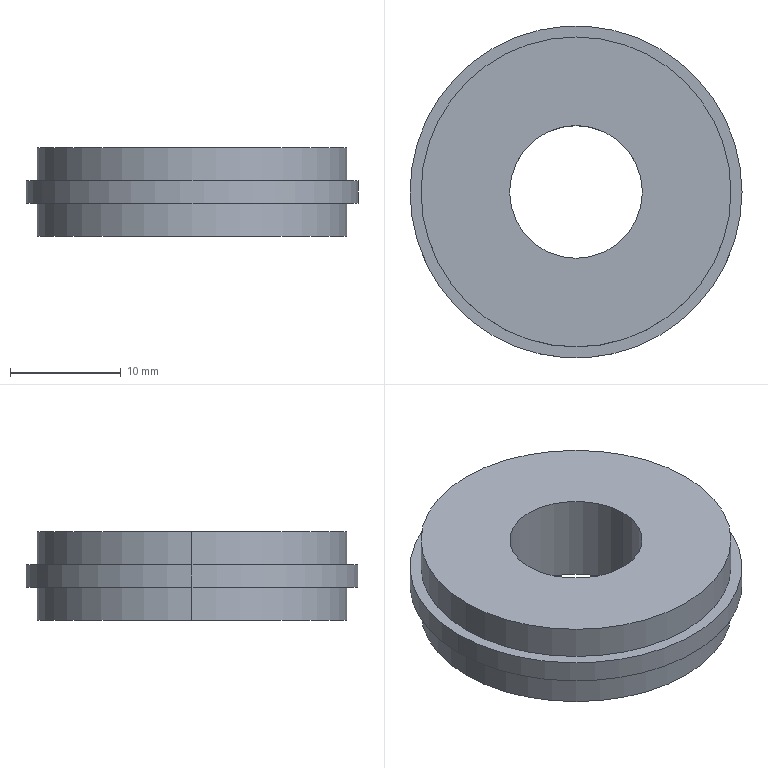Part | SolidWorks | features BaseBody 1 | 1 solid | 12 faces | box 30 x 30 x 8 mm | volume 4203 mm3 | cylinder 8 | plane 4 | commonest cylinder face diameters 28 x4 12 x2 30 x2
STEP:
#1=CARTESIAN_POINT('',(6.,0.,4.));
#2=VERTEX_POINT('',#1);
#3=CARTESIAN_POINT('',(-6.,0.,4.));
#4=VERTEX_POINT('',#3);
#5=CARTESIAN_POINT('',(0.,0.,4.));
#6=DIRECTION('',(0.,0.,-1.));
#7=DIRECTION('',(-1.,0.,0.));
#8=AXIS2_PLACEMENT_3D('',#5,#6,#7);
#9=CIRCLE('',#8,6.);
#10=EDGE_CURVE('',#2,#4,#9,.T.);
#11=ORIENTED_EDGE('',*,*,#10,.F.);
#12=CARTESIAN_POINT('',(6.,0.,-4.));
#13=VERTEX_POINT('',#12);
#14=CARTESIAN_POINT('',(6.,0.,4.));
#15=DIRECTION('',(0.,0.,-1.));
#16=VECTOR('',#15,1000.);
#17=LINE('',#14,#16);
#18=EDGE_CURVE('',#2,#13,#17,.T.);
#19=ORIENTED_EDGE('',*,*,#18,.T.);
#20=CARTESIAN_POINT('',(-6.,0.,-4.));
#21=VERTEX_POINT('',#20);
#22=CARTESIAN_POINT('',(0.,0.,-4.));
#23=DIRECTION('',(0.,0.,-1.));
#24=DIRECTION('',(-1.,0.,0.));
#25=AXIS2_PLACEMENT_3D('',#22,#23,#24);
#26=CIRCLE('',#25,6.);
#27=EDGE_CURVE('',#13,#21,#26,.T.);
#28=ORIENTED_EDGE('',*,*,#27,.T.);
#29=CARTESIAN_POINT('',(-6.,0.,4.));
#30=DIRECTION('',(0.,0.,-1.));
#31=VECTOR('',#30,1000.);
#32=LINE('',#29,#31);
#33=EDGE_CURVE('',#4,#21,#32,.T.);
#34=ORIENTED_EDGE('',*,*,#33,.F.);
#35=EDGE_LOOP('',(#11,#19,#28,#34));
#36=FACE_OUTER_BOUND('',#35,.T.);
#37=CARTESIAN_POINT('',(0.,0.,4.));
#38=DIRECTION('',(0.,0.,-1.));
#39=DIRECTION('',(-1.,0.,0.));
#40=AXIS2_PLACEMENT_3D('',#37,#38,#39);
#41=CYLINDRICAL_SURFACE('',#40,6.);
#42=ADVANCED_FACE('',(#36),#41,.F.);
#43=CARTESIAN_POINT('',(14.,0.,-4.));
#44=VERTEX_POINT('',#43);
#45=CARTESIAN_POINT('',(-14.,0.,-4.));
#46=VERTEX_POINT('',#45);
#47=CARTESIAN_POINT('',(0.,0.,-4.));
#48=DIRECTION('',(0.,0.,1.));
#49=DIRECTION('',(1.,0.,0.));
#50=AXIS2_PLACEMENT_3D('',#47,#48,#49);
#51=CIRCLE('',#50,14.);
#52=EDGE_CURVE('',#44,#46,#51,.T.);
#53=ORIENTED_EDGE('',*,*,#52,.T.);
#54=CARTESIAN_POINT('',(-14.,0.,-1.));
#55=VERTEX_POINT('',#54);
#56=CARTESIAN_POINT('',(-14.,0.,-4.));
#57=DIRECTION('',(0.,0.,1.));
#58=VECTOR('',#57,1000.);
#59=LINE('',#56,#58);
#60=EDGE_CURVE('',#46,#55,#59,.T.);
#61=ORIENTED_EDGE('',*,*,#60,.T.);
#62=CARTESIAN_POINT('',(14.,0.,-1.));
#63=VERTEX_POINT('',#62);
#64=CARTESIAN_POINT('',(0.,0.,-1.));
#65=DIRECTION('',(0.,0.,1.));
#66=DIRECTION('',(1.,0.,0.));
#67=AXIS2_PLACEMENT_3D('',#64,#65,#66);
#68=CIRCLE('',#67,14.);
#69=EDGE_CURVE('',#63,#55,#68,.T.);
#70=ORIENTED_EDGE('',*,*,#69,.F.);
#71=CARTESIAN_POINT('',(14.,0.,-4.));
#72=DIRECTION('',(0.,0.,1.));
#73=VECTOR('',#72,1000.);
#74=LINE('',#71,#73);
#75=EDGE_CURVE('',#44,#63,#74,.T.);
#76=ORIENTED_EDGE('',*,*,#75,.F.);
#77=EDGE_LOOP('',(#53,#61,#70,#76));
#78=FACE_OUTER_BOUND('',#77,.T.);
#79=CARTESIAN_POINT('',(0.,0.,-4.));
#80=DIRECTION('',(0.,0.,1.));
#81=DIRECTION('',(1.,0.,0.));
#82=AXIS2_PLACEMENT_3D('',#79,#80,#81);
#83=CYLINDRICAL_SURFACE('',#82,14.);
#84=ADVANCED_FACE('',(#78),#83,.T.);
#85=CARTESIAN_POINT('',(14.,0.,4.));
#86=VERTEX_POINT('',#85);
#87=CARTESIAN_POINT('',(-14.,0.,4.));
#88=VERTEX_POINT('',#87);
#89=CARTESIAN_POINT('',(0.,0.,4.));
#90=DIRECTION('',(0.,0.,1.));
#91=DIRECTION('',(1.,0.,0.));
#92=AXIS2_PLACEMENT_3D('',#89,#90,#91);
#93=CIRCLE('',#92,14.);
#94=EDGE_CURVE('',#86,#88,#93,.T.);
#95=ORIENTED_EDGE('',*,*,#94,.F.);
#96=CARTESIAN_POINT('',(14.,0.,1.));
#97=VERTEX_POINT('',#96);
#98=CARTESIAN_POINT('',(14.,0.,4.));
#99=DIRECTION('',(0.,0.,-1.));
#100=VECTOR('',#99,1000.);
#101=LINE('',#98,#100);
#102=EDGE_CURVE('',#86,#97,#101,.T.);
#103=ORIENTED_EDGE('',*,*,#102,.T.);
#104=CARTESIAN_POINT('',(-14.,0.,1.));
#105=VERTEX_POINT('',#104);
#106=CARTESIAN_POINT('',(0.,0.,1.));
#107=DIRECTION('',(0.,0.,1.));
#108=DIRECTION('',(1.,0.,0.));
#109=AXIS2_PLACEMENT_3D('',#106,#107,#108);
#110=CIRCLE('',#109,14.);
#111=EDGE_CURVE('',#97,#105,#110,.T.);
#112=ORIENTED_EDGE('',*,*,#111,.T.);
#113=CARTESIAN_POINT('',(-14.,0.,4.));
#114=DIRECTION('',(0.,0.,-1.));
#115=VECTOR('',#114,1000.);
#116=LINE('',#113,#115);
#117=EDGE_CURVE('',#88,#105,#116,.T.);
#118=ORIENTED_EDGE('',*,*,#117,.F.);
#119=EDGE_LOOP('',(#95,#103,#112,#118));
#120=FACE_OUTER_BOUND('',#119,.T.);
#121=CARTESIAN_POINT('',(0.,0.,4.));
#122=DIRECTION('',(0.,0.,-1.));
#123=DIRECTION('',(-1.,0.,0.));
#124=AXIS2_PLACEMENT_3D('',#121,#122,#123);
#125=CYLINDRICAL_SURFACE('',#124,14.);
#126=ADVANCED_FACE('',(#120),#125,.T.);
#127=CARTESIAN_POINT('',(15.,0.,1.));
#128=VERTEX_POINT('',#127);
#129=CARTESIAN_POINT('',(-15.,0.,1.));
#130=VERTEX_POINT('',#129);
#131=CARTESIAN_POINT('',(0.,0.,1.));
#132=DIRECTION('',(0.,0.,1.));
#133=DIRECTION('',(1.,0.,0.));
#134=AXIS2_PLACEMENT_3D('',#131,#132,#133);
#135=CIRCLE('',#134,15.);
#136=EDGE_CURVE('',#128,#130,#135,.T.);
#137=ORIENTED_EDGE('',*,*,#136,.F.);
#138=CARTESIAN_POINT('',(15.,0.,-1.));
#139=VERTEX_POINT('',#138);
#140=CARTESIAN_POINT('',(15.,0.,1.));
#141=DIRECTION('',(0.,0.,-1.));
#142=VECTOR('',#141,1000.);
#143=LINE('',#140,#142);
#144=EDGE_CURVE('',#128,#139,#143,.T.);
#145=ORIENTED_EDGE('',*,*,#144,.T.);
#146=CARTESIAN_POINT('',(-15.,0.,-1.));
#147=VERTEX_POINT('',#146);
#148=CARTESIAN_POINT('',(0.,0.,-1.));
#149=DIRECTION('',(0.,0.,1.));
#150=DIRECTION('',(1.,0.,0.));
#151=AXIS2_PLACEMENT_3D('',#148,#149,#150);
#152=CIRCLE('',#151,15.);
#153=EDGE_CURVE('',#139,#147,#152,.T.);
#154=ORIENTED_EDGE('',*,*,#153,.T.);
#155=CARTESIAN_POINT('',(-15.,0.,1.));
#156=DIRECTION('',(0.,0.,-1.));
#157=VECTOR('',#156,1000.);
#158=LINE('',#155,#157);
#159=EDGE_CURVE('',#130,#147,#158,.T.);
#160=ORIENTED_EDGE('',*,*,#159,.F.);
#161=EDGE_LOOP('',(#137,#145,#154,#160));
#162=FACE_OUTER_BOUND('',#161,.T.);
#163=CARTESIAN_POINT('',(0.,0.,1.));
#164=DIRECTION('',(0.,0.,-1.));
#165=DIRECTION('',(-1.,0.,0.));
#166=AXIS2_PLACEMENT_3D('',#163,#164,#165);
#167=CYLINDRICAL_SURFACE('',#166,15.);
#168=ADVANCED_FACE('',(#162),#167,.T.);
#169=ORIENTED_EDGE('',*,*,#144,.F.);
#170=CARTESIAN_POINT('',(0.,0.,1.));
#171=DIRECTION('',(0.,0.,1.));
#172=DIRECTION('',(1.,0.,0.));
#173=AXIS2_PLACEMENT_3D('',#170,#171,#172);
#174=CIRCLE('',#173,15.);
#175=EDGE_CURVE('',#130,#128,#174,.T.);
#176=ORIENTED_EDGE('',*,*,#175,.F.);
#177=ORIENTED_EDGE('',*,*,#159,.T.);
#178=CARTESIAN_POINT('',(0.,0.,-1.));
#179=DIRECTION('',(0.,0.,1.));
#180=DIRECTION('',(1.,0.,0.));
#181=AXIS2_PLACEMENT_3D('',#178,#179,#180);
#182=CIRCLE('',#181,15.);
#183=EDGE_CURVE('',#147,#139,#182,.T.);
#184=ORIENTED_EDGE('',*,*,#183,.T.);
#185=EDGE_LOOP('',(#169,#176,#177,#184));
#186=FACE_OUTER_BOUND('',#185,.T.);
#187=CARTESIAN_POINT('',(0.,0.,1.));
#188=DIRECTION('',(0.,0.,-1.));
#189=DIRECTION('',(-1.,0.,0.));
#190=AXIS2_PLACEMENT_3D('',#187,#188,#189);
#191=CYLINDRICAL_SURFACE('',#190,15.);
#192=ADVANCED_FACE('',(#186),#191,.T.);
#193=CARTESIAN_POINT('',(0.,0.,1.));
#194=DIRECTION('',(0.,0.,1.));
#195=DIRECTION('',(1.,0.,0.));
#196=AXIS2_PLACEMENT_3D('',#193,#194,#195);
#197=CIRCLE('',#196,14.);
#198=EDGE_CURVE('',#105,#97,#197,.T.);
#199=ORIENTED_EDGE('',*,*,#198,.F.);
#200=ORIENTED_EDGE('',*,*,#111,.F.);
#201=EDGE_LOOP('',(#199,#200));
#202=FACE_BOUND('',#201,.T.);
#203=ORIENTED_EDGE('',*,*,#175,.T.);
#204=ORIENTED_EDGE('',*,*,#136,.T.);
#205=EDGE_LOOP('',(#203,#204));
#206=FACE_OUTER_BOUND('',#205,.T.);
#207=CARTESIAN_POINT('',(0.,0.,1.));
#208=DIRECTION('',(0.,0.,1.));
#209=DIRECTION('',(1.,0.,0.));
#210=AXIS2_PLACEMENT_3D('',#207,#208,#209);
#211=PLANE('',#210);
#212=ADVANCED_FACE('',(#202,#206),#211,.T.);
#213=ORIENTED_EDGE('',*,*,#69,.T.);
#214=CARTESIAN_POINT('',(0.,0.,-1.));
#215=DIRECTION('',(0.,0.,1.));
#216=DIRECTION('',(1.,0.,0.));
#217=AXIS2_PLACEMENT_3D('',#214,#215,#216);
#218=CIRCLE('',#217,14.);
#219=EDGE_CURVE('',#55,#63,#218,.T.);
#220=ORIENTED_EDGE('',*,*,#219,.T.);
#221=EDGE_LOOP('',(#213,#220));
#222=FACE_BOUND('',#221,.T.);
#223=ORIENTED_EDGE('',*,*,#183,.F.);
#224=ORIENTED_EDGE('',*,*,#153,.F.);
#225=EDGE_LOOP('',(#223,#224));
#226=FACE_OUTER_BOUND('',#225,.T.);
#227=CARTESIAN_POINT('',(0.,0.,-1.));
#228=DIRECTION('',(0.,0.,1.));
#229=DIRECTION('',(1.,0.,0.));
#230=AXIS2_PLACEMENT_3D('',#227,#228,#229);
#231=PLANE('',#230);
#232=ADVANCED_FACE('',(#222,#226),#231,.F.);
#233=ORIENTED_EDGE('',*,*,#102,.F.);
#234=CARTESIAN_POINT('',(0.,0.,4.));
#235=DIRECTION('',(0.,0.,1.));
#236=DIRECTION('',(1.,0.,0.));
#237=AXIS2_PLACEMENT_3D('',#234,#235,#236);
#238=CIRCLE('',#237,14.);
#239=EDGE_CURVE('',#88,#86,#238,.T.);
#240=ORIENTED_EDGE('',*,*,#239,.F.);
#241=ORIENTED_EDGE('',*,*,#117,.T.);
#242=ORIENTED_EDGE('',*,*,#198,.T.);
#243=EDGE_LOOP('',(#233,#240,#241,#242));
#244=FACE_OUTER_BOUND('',#243,.T.);
#245=CARTESIAN_POINT('',(0.,0.,4.));
#246=DIRECTION('',(0.,0.,-1.));
#247=DIRECTION('',(-1.,0.,0.));
#248=AXIS2_PLACEMENT_3D('',#245,#246,#247);
#249=CYLINDRICAL_SURFACE('',#248,14.);
#250=ADVANCED_FACE('',(#244),#249,.T.);
#251=CARTESIAN_POINT('',(0.,0.,4.));
#252=DIRECTION('',(0.,0.,-1.));
#253=DIRECTION('',(-1.,0.,0.));
#254=AXIS2_PLACEMENT_3D('',#251,#252,#253);
#255=CIRCLE('',#254,6.);
#256=EDGE_CURVE('',#4,#2,#255,.T.);
#257=ORIENTED_EDGE('',*,*,#256,.T.);
#258=ORIENTED_EDGE('',*,*,#10,.T.);
#259=EDGE_LOOP('',(#257,#258));
#260=FACE_BOUND('',#259,.T.);
#261=ORIENTED_EDGE('',*,*,#239,.T.);
#262=ORIENTED_EDGE('',*,*,#94,.T.);
#263=EDGE_LOOP('',(#261,#262));
#264=FACE_OUTER_BOUND('',#263,.T.);
#265=CARTESIAN_POINT('',(0.,0.,4.));
#266=DIRECTION('',(0.,0.,1.));
#267=DIRECTION('',(1.,0.,0.));
#268=AXIS2_PLACEMENT_3D('',#265,#266,#267);
#269=PLANE('',#268);
#270=ADVANCED_FACE('',(#260,#264),#269,.T.);
#271=ORIENTED_EDGE('',*,*,#60,.F.);
#272=CARTESIAN_POINT('',(0.,0.,-4.));
#273=DIRECTION('',(0.,0.,1.));
#274=DIRECTION('',(1.,0.,0.));
#275=AXIS2_PLACEMENT_3D('',#272,#273,#274);
#276=CIRCLE('',#275,14.);
#277=EDGE_CURVE('',#46,#44,#276,.T.);
#278=ORIENTED_EDGE('',*,*,#277,.T.);
#279=ORIENTED_EDGE('',*,*,#75,.T.);
#280=ORIENTED_EDGE('',*,*,#219,.F.);
#281=EDGE_LOOP('',(#271,#278,#279,#280));
#282=FACE_OUTER_BOUND('',#281,.T.);
#283=CARTESIAN_POINT('',(0.,0.,-4.));
#284=DIRECTION('',(0.,0.,1.));
#285=DIRECTION('',(1.,0.,0.));
#286=AXIS2_PLACEMENT_3D('',#283,#284,#285);
#287=CYLINDRICAL_SURFACE('',#286,14.);
#288=ADVANCED_FACE('',(#282),#287,.T.);
#289=CARTESIAN_POINT('',(0.,0.,-4.));
#290=DIRECTION('',(0.,0.,-1.));
#291=DIRECTION('',(-1.,0.,0.));
#292=AXIS2_PLACEMENT_3D('',#289,#290,#291);
#293=CIRCLE('',#292,6.);
#294=EDGE_CURVE('',#21,#13,#293,.T.);
#295=ORIENTED_EDGE('',*,*,#294,.F.);
#296=ORIENTED_EDGE('',*,*,#27,.F.);
#297=EDGE_LOOP('',(#295,#296));
#298=FACE_BOUND('',#297,.T.);
#299=ORIENTED_EDGE('',*,*,#52,.F.);
#300=ORIENTED_EDGE('',*,*,#277,.F.);
#301=EDGE_LOOP('',(#299,#300));
#302=FACE_OUTER_BOUND('',#301,.T.);
#303=CARTESIAN_POINT('',(0.,0.,-4.));
#304=DIRECTION('',(0.,0.,-1.));
#305=DIRECTION('',(1.,0.,0.));
#306=AXIS2_PLACEMENT_3D('',#303,#304,#305);
#307=PLANE('',#306);
#308=ADVANCED_FACE('',(#298,#302),#307,.T.);
#309=ORIENTED_EDGE('',*,*,#18,.F.);
#310=ORIENTED_EDGE('',*,*,#256,.F.);
#311=ORIENTED_EDGE('',*,*,#33,.T.);
#312=ORIENTED_EDGE('',*,*,#294,.T.);
#313=EDGE_LOOP('',(#309,#310,#311,#312));
#314=FACE_OUTER_BOUND('',#313,.T.);
#315=CARTESIAN_POINT('',(0.,0.,4.));
#316=DIRECTION('',(0.,0.,-1.));
#317=DIRECTION('',(-1.,0.,0.));
#318=AXIS2_PLACEMENT_3D('',#315,#316,#317);
#319=CYLINDRICAL_SURFACE('',#318,6.);
#320=ADVANCED_FACE('',(#314),#319,.F.);
#321=CLOSED_SHELL('',(#42,#84,#126,#168,#192,#212,#232,#250,#270,#288,#308,#320));
#322=MANIFOLD_SOLID_BREP('',#321);
#323=CARTESIAN_POINT('',(0.,0.,0.));
#324=DIRECTION('',(0.,0.,1.));
#325=DIRECTION('',(1.,0.,0.));
#326=AXIS2_PLACEMENT_3D('',#323,#324,#325);
#327=(LENGTH_UNIT()NAMED_UNIT(*)SI_UNIT(.MILLI.,.METRE.));
#328=UNCERTAINTY_MEASURE_WITH_UNIT(LENGTH_MEASURE(0.00001),#327,'','');
#329=(NAMED_UNIT(*)PLANE_ANGLE_UNIT()SI_UNIT($,.RADIAN.));
#330=(NAMED_UNIT(*)SI_UNIT($,.STERADIAN.)SOLID_ANGLE_UNIT());
#331=(GEOMETRIC_REPRESENTATION_CONTEXT(3)GLOBAL_UNCERTAINTY_ASSIGNED_CONTEXT((#328))GLOBAL_UNIT_ASSIGNED_CONTEXT((#327,#329,#330))REPRESENTATION_CONTEXT('',''));
#332=ADVANCED_BREP_SHAPE_REPRESENTATION('',(#322,#326),#331);